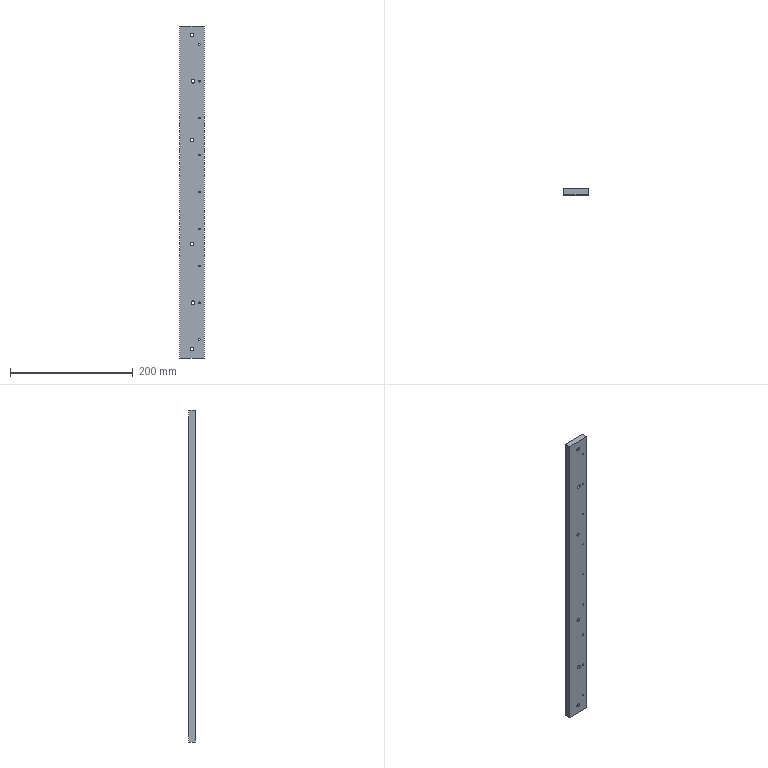Part | STEP file | 0245_218_Plate | 1 solid | 48 faces | box 40 x 10 x 540 mm | volume 212947 mm3 | cylinder 38 | plane 10 | commonest cylinder face diameters 2.5 x18 5.5 x8 10 x8 6 x4